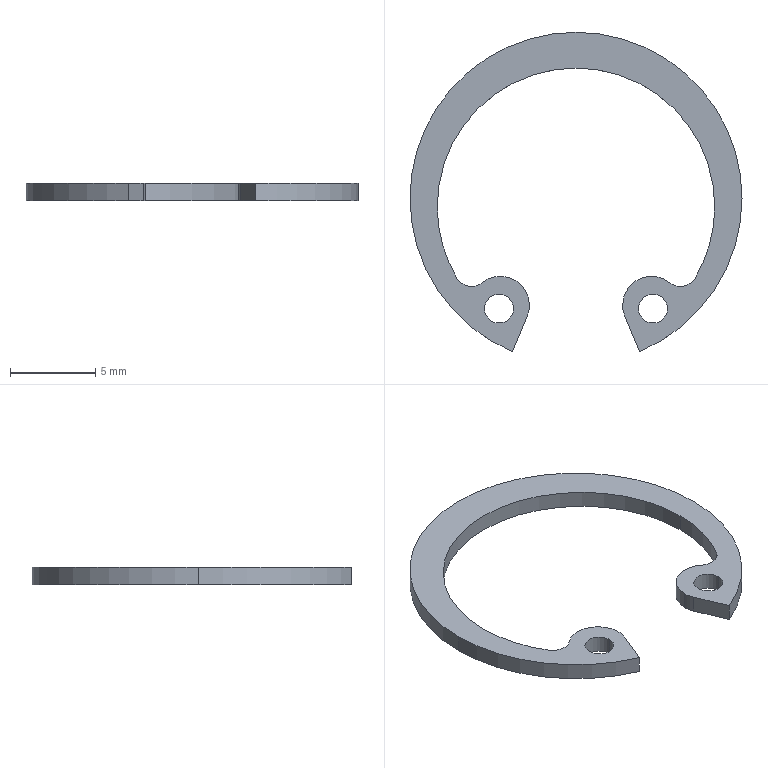Part | SolidWorks | features Extrusion 1 | 1 solid | 19 faces | box 19.5 x 18.758 x 1 mm | volume 92.859 mm3 | cylinder 15 | plane 4 | commonest cylinder face diameters 1.7 x4 3.4 x3 16.3 x3 19.5 x3 2 x2
STEP:
#1=CARTESIAN_POINT('',(3.673,-6.477,1.));
#2=VERTEX_POINT('',#1);
#3=CARTESIAN_POINT('',(5.373,-6.477,1.));
#4=VERTEX_POINT('',#3);
#5=CARTESIAN_POINT('',(4.523,-6.477,1.));
#6=DIRECTION('',(0.,0.,1.));
#7=DIRECTION('',(-1.,0.,0.));
#8=AXIS2_PLACEMENT_3D('',#5,#6,#7);
#9=CIRCLE('',#8,0.85);
#10=EDGE_CURVE('',#2,#4,#9,.T.);
#11=ORIENTED_EDGE('',*,*,#10,.T.);
#12=CARTESIAN_POINT('',(5.373,-6.477,0.));
#13=VERTEX_POINT('',#12);
#14=CARTESIAN_POINT('',(5.373,-6.477,1.));
#15=DIRECTION('',(0.,0.,-1.));
#16=VECTOR('',#15,1000.);
#17=LINE('',#14,#16);
#18=EDGE_CURVE('',#4,#13,#17,.T.);
#19=ORIENTED_EDGE('',*,*,#18,.T.);
#20=CARTESIAN_POINT('',(3.673,-6.477,0.));
#21=VERTEX_POINT('',#20);
#22=CARTESIAN_POINT('',(4.523,-6.477,0.));
#23=DIRECTION('',(0.,0.,1.));
#24=DIRECTION('',(-1.,0.,0.));
#25=AXIS2_PLACEMENT_3D('',#22,#23,#24);
#26=CIRCLE('',#25,0.85);
#27=EDGE_CURVE('',#21,#13,#26,.T.);
#28=ORIENTED_EDGE('',*,*,#27,.F.);
#29=CARTESIAN_POINT('',(3.673,-6.477,1.));
#30=DIRECTION('',(0.,0.,-1.));
#31=VECTOR('',#30,1000.);
#32=LINE('',#29,#31);
#33=EDGE_CURVE('',#2,#21,#32,.T.);
#34=ORIENTED_EDGE('',*,*,#33,.F.);
#35=EDGE_LOOP('',(#11,#19,#28,#34));
#36=FACE_OUTER_BOUND('',#35,.T.);
#37=CARTESIAN_POINT('',(4.523,-6.477,1.));
#38=DIRECTION('',(0.,0.,-1.));
#39=DIRECTION('',(-1.,0.,0.));
#40=AXIS2_PLACEMENT_3D('',#37,#38,#39);
#41=CYLINDRICAL_SURFACE('',#40,0.85);
#42=ADVANCED_FACE('',(#36),#41,.F.);
#43=CARTESIAN_POINT('',(-5.373,-6.477,1.));
#44=VERTEX_POINT('',#43);
#45=CARTESIAN_POINT('',(-3.673,-6.477,1.));
#46=VERTEX_POINT('',#45);
#47=CARTESIAN_POINT('',(-4.523,-6.477,1.));
#48=DIRECTION('',(0.,0.,1.));
#49=DIRECTION('',(1.,0.,0.));
#50=AXIS2_PLACEMENT_3D('',#47,#48,#49);
#51=CIRCLE('',#50,0.85);
#52=EDGE_CURVE('',#44,#46,#51,.T.);
#53=ORIENTED_EDGE('',*,*,#52,.T.);
#54=CARTESIAN_POINT('',(-3.673,-6.477,0.));
#55=VERTEX_POINT('',#54);
#56=CARTESIAN_POINT('',(-3.673,-6.477,1.));
#57=DIRECTION('',(0.,0.,-1.));
#58=VECTOR('',#57,1000.);
#59=LINE('',#56,#58);
#60=EDGE_CURVE('',#46,#55,#59,.T.);
#61=ORIENTED_EDGE('',*,*,#60,.T.);
#62=CARTESIAN_POINT('',(-5.373,-6.477,0.));
#63=VERTEX_POINT('',#62);
#64=CARTESIAN_POINT('',(-4.523,-6.477,0.));
#65=DIRECTION('',(0.,0.,1.));
#66=DIRECTION('',(1.,0.,0.));
#67=AXIS2_PLACEMENT_3D('',#64,#65,#66);
#68=CIRCLE('',#67,0.85);
#69=EDGE_CURVE('',#63,#55,#68,.T.);
#70=ORIENTED_EDGE('',*,*,#69,.F.);
#71=CARTESIAN_POINT('',(-5.373,-6.477,1.));
#72=DIRECTION('',(0.,0.,-1.));
#73=VECTOR('',#72,1000.);
#74=LINE('',#71,#73);
#75=EDGE_CURVE('',#44,#63,#74,.T.);
#76=ORIENTED_EDGE('',*,*,#75,.F.);
#77=EDGE_LOOP('',(#53,#61,#70,#76));
#78=FACE_OUTER_BOUND('',#77,.T.);
#79=CARTESIAN_POINT('',(-4.523,-6.477,1.));
#80=DIRECTION('',(0.,0.,-1.));
#81=DIRECTION('',(-1.,0.,0.));
#82=AXIS2_PLACEMENT_3D('',#79,#80,#81);
#83=CYLINDRICAL_SURFACE('',#82,0.85);
#84=ADVANCED_FACE('',(#78),#83,.F.);
#85=CARTESIAN_POINT('',(9.75,0.,1.));
#86=VERTEX_POINT('',#85);
#87=CARTESIAN_POINT('',(-9.75,0.,1.));
#88=VERTEX_POINT('',#87);
#89=CARTESIAN_POINT('',(0.,0.,1.));
#90=DIRECTION('',(0.,0.,1.));
#91=DIRECTION('',(1.,0.,0.));
#92=AXIS2_PLACEMENT_3D('',#89,#90,#91);
#93=CIRCLE('',#92,9.75);
#94=EDGE_CURVE('',#86,#88,#93,.T.);
#95=ORIENTED_EDGE('',*,*,#94,.F.);
#96=CARTESIAN_POINT('',(9.75,0.,0.));
#97=VERTEX_POINT('',#96);
#98=CARTESIAN_POINT('',(9.75,0.,1.));
#99=DIRECTION('',(0.,0.,-1.));
#100=VECTOR('',#99,1000.);
#101=LINE('',#98,#100);
#102=EDGE_CURVE('',#86,#97,#101,.T.);
#103=ORIENTED_EDGE('',*,*,#102,.T.);
#104=CARTESIAN_POINT('',(-9.75,0.,0.));
#105=VERTEX_POINT('',#104);
#106=CARTESIAN_POINT('',(0.,0.,0.));
#107=DIRECTION('',(0.,0.,1.));
#108=DIRECTION('',(1.,0.,0.));
#109=AXIS2_PLACEMENT_3D('',#106,#107,#108);
#110=CIRCLE('',#109,9.75);
#111=EDGE_CURVE('',#97,#105,#110,.T.);
#112=ORIENTED_EDGE('',*,*,#111,.T.);
#113=CARTESIAN_POINT('',(-9.75,0.,1.));
#114=DIRECTION('',(0.,0.,-1.));
#115=VECTOR('',#114,1000.);
#116=LINE('',#113,#115);
#117=EDGE_CURVE('',#88,#105,#116,.T.);
#118=ORIENTED_EDGE('',*,*,#117,.F.);
#119=EDGE_LOOP('',(#95,#103,#112,#118));
#120=FACE_OUTER_BOUND('',#119,.T.);
#121=CARTESIAN_POINT('',(0.,0.,1.));
#122=DIRECTION('',(0.,0.,-1.));
#123=DIRECTION('',(-1.,0.,0.));
#124=AXIS2_PLACEMENT_3D('',#121,#122,#123);
#125=CYLINDRICAL_SURFACE('',#124,9.75);
#126=ADVANCED_FACE('',(#120),#125,.T.);
#127=CARTESIAN_POINT('',(-3.731,-9.008,1.));
#128=VERTEX_POINT('',#127);
#129=CARTESIAN_POINT('',(0.,0.,1.));
#130=DIRECTION('',(0.,0.,1.));
#131=DIRECTION('',(1.,0.,0.));
#132=AXIS2_PLACEMENT_3D('',#129,#130,#131);
#133=CIRCLE('',#132,9.75);
#134=EDGE_CURVE('',#88,#128,#133,.T.);
#135=ORIENTED_EDGE('',*,*,#134,.F.);
#136=ORIENTED_EDGE('',*,*,#117,.T.);
#137=CARTESIAN_POINT('',(-3.731,-9.008,0.));
#138=VERTEX_POINT('',#137);
#139=CARTESIAN_POINT('',(0.,0.,0.));
#140=DIRECTION('',(0.,0.,1.));
#141=DIRECTION('',(1.,0.,0.));
#142=AXIS2_PLACEMENT_3D('',#139,#140,#141);
#143=CIRCLE('',#142,9.75);
#144=EDGE_CURVE('',#105,#138,#143,.T.);
#145=ORIENTED_EDGE('',*,*,#144,.T.);
#146=CARTESIAN_POINT('',(-3.731,-9.008,1.));
#147=DIRECTION('',(0.,0.,-1.));
#148=VECTOR('',#147,1000.);
#149=LINE('',#146,#148);
#150=EDGE_CURVE('',#128,#138,#149,.T.);
#151=ORIENTED_EDGE('',*,*,#150,.F.);
#152=EDGE_LOOP('',(#135,#136,#145,#151));
#153=FACE_OUTER_BOUND('',#152,.T.);
#154=CARTESIAN_POINT('',(0.,0.,1.));
#155=DIRECTION('',(0.,0.,-1.));
#156=DIRECTION('',(-1.,0.,0.));
#157=AXIS2_PLACEMENT_3D('',#154,#155,#156);
#158=CYLINDRICAL_SURFACE('',#157,9.75);
#159=ADVANCED_FACE('',(#153),#158,.T.);
#160=CARTESIAN_POINT('',(2.741,-6.278,1.));
#161=VERTEX_POINT('',#160);
#162=CARTESIAN_POINT('',(2.87,-6.929,1.));
#163=VERTEX_POINT('',#162);
#164=CARTESIAN_POINT('',(4.441,-6.278,1.));
#165=DIRECTION('',(0.,0.,1.));
#166=DIRECTION('',(-1.,0.,0.));
#167=AXIS2_PLACEMENT_3D('',#164,#165,#166);
#168=CIRCLE('',#167,1.7);
#169=EDGE_CURVE('',#161,#163,#168,.T.);
#170=ORIENTED_EDGE('',*,*,#169,.F.);
#171=CARTESIAN_POINT('',(2.741,-6.278,0.));
#172=VERTEX_POINT('',#171);
#173=CARTESIAN_POINT('',(2.741,-6.278,1.));
#174=DIRECTION('',(0.,0.,-1.));
#175=VECTOR('',#174,1000.);
#176=LINE('',#173,#175);
#177=EDGE_CURVE('',#161,#172,#176,.T.);
#178=ORIENTED_EDGE('',*,*,#177,.T.);
#179=CARTESIAN_POINT('',(2.87,-6.929,0.));
#180=VERTEX_POINT('',#179);
#181=CARTESIAN_POINT('',(4.441,-6.278,0.));
#182=DIRECTION('',(0.,0.,1.));
#183=DIRECTION('',(-1.,0.,0.));
#184=AXIS2_PLACEMENT_3D('',#181,#182,#183);
#185=CIRCLE('',#184,1.7);
#186=EDGE_CURVE('',#172,#180,#185,.T.);
#187=ORIENTED_EDGE('',*,*,#186,.T.);
#188=CARTESIAN_POINT('',(2.87,-6.929,1.));
#189=DIRECTION('',(0.,0.,-1.));
#190=VECTOR('',#189,1000.);
#191=LINE('',#188,#190);
#192=EDGE_CURVE('',#163,#180,#191,.T.);
#193=ORIENTED_EDGE('',*,*,#192,.F.);
#194=EDGE_LOOP('',(#170,#178,#187,#193));
#195=FACE_OUTER_BOUND('',#194,.T.);
#196=CARTESIAN_POINT('',(4.441,-6.278,1.));
#197=DIRECTION('',(0.,0.,-1.));
#198=DIRECTION('',(-1.,0.,0.));
#199=AXIS2_PLACEMENT_3D('',#196,#197,#198);
#200=CYLINDRICAL_SURFACE('',#199,1.7);
#201=ADVANCED_FACE('',(#195),#200,.T.);
#202=CARTESIAN_POINT('',(8.15,-0.5,1.));
#203=VERTEX_POINT('',#202);
#204=CARTESIAN_POINT('',(6.991,-4.689,1.));
#205=VERTEX_POINT('',#204);
#206=CARTESIAN_POINT('',(0.,-0.5,1.));
#207=DIRECTION('',(0.,0.,-1.));
#208=DIRECTION('',(1.,0.,0.));
#209=AXIS2_PLACEMENT_3D('',#206,#207,#208);
#210=CIRCLE('',#209,8.15);
#211=EDGE_CURVE('',#203,#205,#210,.T.);
#212=ORIENTED_EDGE('',*,*,#211,.F.);
#213=CARTESIAN_POINT('',(8.15,-0.5,0.));
#214=VERTEX_POINT('',#213);
#215=CARTESIAN_POINT('',(8.15,-0.5,1.));
#216=DIRECTION('',(0.,0.,-1.));
#217=VECTOR('',#216,1000.);
#218=LINE('',#215,#217);
#219=EDGE_CURVE('',#203,#214,#218,.T.);
#220=ORIENTED_EDGE('',*,*,#219,.T.);
#221=CARTESIAN_POINT('',(6.991,-4.689,0.));
#222=VERTEX_POINT('',#221);
#223=CARTESIAN_POINT('',(0.,-0.5,0.));
#224=DIRECTION('',(0.,0.,-1.));
#225=DIRECTION('',(1.,0.,0.));
#226=AXIS2_PLACEMENT_3D('',#223,#224,#225);
#227=CIRCLE('',#226,8.15);
#228=EDGE_CURVE('',#214,#222,#227,.T.);
#229=ORIENTED_EDGE('',*,*,#228,.T.);
#230=CARTESIAN_POINT('',(6.991,-4.689,1.));
#231=DIRECTION('',(0.,0.,-1.));
#232=VECTOR('',#231,1000.);
#233=LINE('',#230,#232);
#234=EDGE_CURVE('',#205,#222,#233,.T.);
#235=ORIENTED_EDGE('',*,*,#234,.F.);
#236=EDGE_LOOP('',(#212,#220,#229,#235));
#237=FACE_OUTER_BOUND('',#236,.T.);
#238=CARTESIAN_POINT('',(0.,-0.5,1.));
#239=DIRECTION('',(0.,0.,-1.));
#240=DIRECTION('',(-1.,0.,0.));
#241=AXIS2_PLACEMENT_3D('',#238,#239,#240);
#242=CYLINDRICAL_SURFACE('',#241,8.15);
#243=ADVANCED_FACE('',(#237),#242,.F.);
#244=ORIENTED_EDGE('',*,*,#219,.F.);
#245=CARTESIAN_POINT('',(-8.15,-0.5,1.));
#246=VERTEX_POINT('',#245);
#247=CARTESIAN_POINT('',(0.,-0.5,1.));
#248=DIRECTION('',(0.,0.,-1.));
#249=DIRECTION('',(1.,0.,0.));
#250=AXIS2_PLACEMENT_3D('',#247,#248,#249);
#251=CIRCLE('',#250,8.15);
#252=EDGE_CURVE('',#246,#203,#251,.T.);
#253=ORIENTED_EDGE('',*,*,#252,.F.);
#254=CARTESIAN_POINT('',(-8.15,-0.5,0.));
#255=VERTEX_POINT('',#254);
#256=CARTESIAN_POINT('',(-8.15,-0.5,1.));
#257=DIRECTION('',(0.,0.,-1.));
#258=VECTOR('',#257,1000.);
#259=LINE('',#256,#258);
#260=EDGE_CURVE('',#246,#255,#259,.T.);
#261=ORIENTED_EDGE('',*,*,#260,.T.);
#262=CARTESIAN_POINT('',(0.,-0.5,0.));
#263=DIRECTION('',(0.,0.,-1.));
#264=DIRECTION('',(1.,0.,0.));
#265=AXIS2_PLACEMENT_3D('',#262,#263,#264);
#266=CIRCLE('',#265,8.15);
#267=EDGE_CURVE('',#255,#214,#266,.T.);
#268=ORIENTED_EDGE('',*,*,#267,.T.);
#269=EDGE_LOOP('',(#244,#253,#261,#268));
#270=FACE_OUTER_BOUND('',#269,.T.);
#271=CARTESIAN_POINT('',(0.,-0.5,1.));
#272=DIRECTION('',(0.,0.,-1.));
#273=DIRECTION('',(-1.,0.,0.));
#274=AXIS2_PLACEMENT_3D('',#271,#272,#273);
#275=CYLINDRICAL_SURFACE('',#274,8.15);
#276=ADVANCED_FACE('',(#270),#275,.F.);
#277=ORIENTED_EDGE('',*,*,#52,.F.);
#278=CARTESIAN_POINT('',(-4.523,-6.477,1.));
#279=DIRECTION('',(0.,0.,1.));
#280=DIRECTION('',(1.,0.,0.));
#281=AXIS2_PLACEMENT_3D('',#278,#279,#280);
#282=CIRCLE('',#281,0.85);
#283=EDGE_CURVE('',#46,#44,#282,.T.);
#284=ORIENTED_EDGE('',*,*,#283,.F.);
#285=EDGE_LOOP('',(#277,#284));
#286=FACE_BOUND('',#285,.T.);
#287=CARTESIAN_POINT('',(-2.87,-6.929,1.));
#288=VERTEX_POINT('',#287);
#289=CARTESIAN_POINT('',(-5.506,-4.954,1.));
#290=VERTEX_POINT('',#289);
#291=CARTESIAN_POINT('',(-4.441,-6.278,1.));
#292=DIRECTION('',(0.,0.,1.));
#293=DIRECTION('',(1.,0.,0.));
#294=AXIS2_PLACEMENT_3D('',#291,#292,#293);
#295=CIRCLE('',#294,1.7);
#296=EDGE_CURVE('',#288,#290,#295,.T.);
#297=ORIENTED_EDGE('',*,*,#296,.T.);
#298=CARTESIAN_POINT('',(-6.991,-4.689,1.));
#299=VERTEX_POINT('',#298);
#300=CARTESIAN_POINT('',(-6.133,-4.175,1.));
#301=DIRECTION('',(0.,0.,-1.));
#302=DIRECTION('',(-1.,0.,0.));
#303=AXIS2_PLACEMENT_3D('',#300,#301,#302);
#304=CIRCLE('',#303,1.);
#305=EDGE_CURVE('',#290,#299,#304,.T.);
#306=ORIENTED_EDGE('',*,*,#305,.T.);
#307=CARTESIAN_POINT('',(0.,-0.5,1.));
#308=DIRECTION('',(0.,0.,-1.));
#309=DIRECTION('',(1.,0.,0.));
#310=AXIS2_PLACEMENT_3D('',#307,#308,#309);
#311=CIRCLE('',#310,8.15);
#312=EDGE_CURVE('',#299,#246,#311,.T.);
#313=ORIENTED_EDGE('',*,*,#312,.T.);
#314=ORIENTED_EDGE('',*,*,#252,.T.);
#315=ORIENTED_EDGE('',*,*,#211,.T.);
#316=CARTESIAN_POINT('',(5.506,-4.954,1.));
#317=VERTEX_POINT('',#316);
#318=CARTESIAN_POINT('',(6.133,-4.175,1.));
#319=DIRECTION('',(0.,0.,-1.));
#320=DIRECTION('',(1.,0.,0.));
#321=AXIS2_PLACEMENT_3D('',#318,#319,#320);
#322=CIRCLE('',#321,1.);
#323=EDGE_CURVE('',#205,#317,#322,.T.);
#324=ORIENTED_EDGE('',*,*,#323,.T.);
#325=CARTESIAN_POINT('',(4.441,-6.278,1.));
#326=DIRECTION('',(0.,0.,1.));
#327=DIRECTION('',(-1.,0.,0.));
#328=AXIS2_PLACEMENT_3D('',#325,#326,#327);
#329=CIRCLE('',#328,1.7);
#330=EDGE_CURVE('',#317,#161,#329,.T.);
#331=ORIENTED_EDGE('',*,*,#330,.T.);
#332=ORIENTED_EDGE('',*,*,#169,.T.);
#333=CARTESIAN_POINT('',(3.731,-9.008,1.));
#334=VERTEX_POINT('',#333);
#335=CARTESIAN_POINT('',(2.87,-6.929,1.));
#336=DIRECTION('',(0.3827,-0.9239,0.));
#337=VECTOR('',#336,1000.);
#338=LINE('',#335,#337);
#339=EDGE_CURVE('',#163,#334,#338,.T.);
#340=ORIENTED_EDGE('',*,*,#339,.T.);
#341=CARTESIAN_POINT('',(0.,0.,1.));
#342=DIRECTION('',(0.,0.,1.));
#343=DIRECTION('',(1.,0.,0.));
#344=AXIS2_PLACEMENT_3D('',#341,#342,#343);
#345=CIRCLE('',#344,9.75);
#346=EDGE_CURVE('',#334,#86,#345,.T.);
#347=ORIENTED_EDGE('',*,*,#346,.T.);
#348=ORIENTED_EDGE('',*,*,#94,.T.);
#349=ORIENTED_EDGE('',*,*,#134,.T.);
#350=CARTESIAN_POINT('',(-2.87,-6.929,1.));
#351=DIRECTION('',(0.3827,0.9239,0.));
#352=VECTOR('',#351,1000.);
#353=LINE('',#350,#352);
#354=EDGE_CURVE('',#128,#288,#353,.T.);
#355=ORIENTED_EDGE('',*,*,#354,.T.);
#356=EDGE_LOOP('',(#297,#306,#313,#314,#315,#324,#331,#332,#340,#347,#348,#349,#355));
#357=FACE_OUTER_BOUND('',#356,.T.);
#358=ORIENTED_EDGE('',*,*,#10,.F.);
#359=CARTESIAN_POINT('',(4.523,-6.477,1.));
#360=DIRECTION('',(0.,0.,1.));
#361=DIRECTION('',(-1.,0.,0.));
#362=AXIS2_PLACEMENT_3D('',#359,#360,#361);
#363=CIRCLE('',#362,0.85);
#364=EDGE_CURVE('',#4,#2,#363,.T.);
#365=ORIENTED_EDGE('',*,*,#364,.F.);
#366=EDGE_LOOP('',(#358,#365));
#367=FACE_BOUND('',#366,.T.);
#368=CARTESIAN_POINT('',(-4.441,-6.278,1.));
#369=DIRECTION('',(0.,0.,1.));
#370=DIRECTION('',(1.,0.,0.));
#371=AXIS2_PLACEMENT_3D('',#368,#369,#370);
#372=PLANE('',#371);
#373=ADVANCED_FACE('',(#286,#357,#367),#372,.T.);
#374=CARTESIAN_POINT('',(-2.87,-6.929,0.));
#375=VERTEX_POINT('',#374);
#376=CARTESIAN_POINT('',(-5.506,-4.954,0.));
#377=VERTEX_POINT('',#376);
#378=CARTESIAN_POINT('',(-4.441,-6.278,0.));
#379=DIRECTION('',(0.,0.,1.));
#380=DIRECTION('',(1.,0.,0.));
#381=AXIS2_PLACEMENT_3D('',#378,#379,#380);
#382=CIRCLE('',#381,1.7);
#383=EDGE_CURVE('',#375,#377,#382,.T.);
#384=ORIENTED_EDGE('',*,*,#383,.F.);
#385=CARTESIAN_POINT('',(-2.87,-6.929,0.));
#386=DIRECTION('',(0.3827,0.9239,0.));
#387=VECTOR('',#386,1000.);
#388=LINE('',#385,#387);
#389=EDGE_CURVE('',#138,#375,#388,.T.);
#390=ORIENTED_EDGE('',*,*,#389,.F.);
#391=ORIENTED_EDGE('',*,*,#144,.F.);
#392=ORIENTED_EDGE('',*,*,#111,.F.);
#393=CARTESIAN_POINT('',(3.731,-9.008,0.));
#394=VERTEX_POINT('',#393);
#395=CARTESIAN_POINT('',(0.,0.,0.));
#396=DIRECTION('',(0.,0.,1.));
#397=DIRECTION('',(1.,0.,0.));
#398=AXIS2_PLACEMENT_3D('',#395,#396,#397);
#399=CIRCLE('',#398,9.75);
#400=EDGE_CURVE('',#394,#97,#399,.T.);
#401=ORIENTED_EDGE('',*,*,#400,.F.);
#402=CARTESIAN_POINT('',(2.87,-6.929,0.));
#403=DIRECTION('',(0.3827,-0.9239,0.));
#404=VECTOR('',#403,1000.);
#405=LINE('',#402,#404);
#406=EDGE_CURVE('',#180,#394,#405,.T.);
#407=ORIENTED_EDGE('',*,*,#406,.F.);
#408=ORIENTED_EDGE('',*,*,#186,.F.);
#409=CARTESIAN_POINT('',(5.506,-4.954,0.));
#410=VERTEX_POINT('',#409);
#411=CARTESIAN_POINT('',(4.441,-6.278,0.));
#412=DIRECTION('',(0.,0.,1.));
#413=DIRECTION('',(-1.,0.,0.));
#414=AXIS2_PLACEMENT_3D('',#411,#412,#413);
#415=CIRCLE('',#414,1.7);
#416=EDGE_CURVE('',#410,#172,#415,.T.);
#417=ORIENTED_EDGE('',*,*,#416,.F.);
#418=CARTESIAN_POINT('',(6.133,-4.175,0.));
#419=DIRECTION('',(0.,0.,-1.));
#420=DIRECTION('',(1.,0.,0.));
#421=AXIS2_PLACEMENT_3D('',#418,#419,#420);
#422=CIRCLE('',#421,1.);
#423=EDGE_CURVE('',#222,#410,#422,.T.);
#424=ORIENTED_EDGE('',*,*,#423,.F.);
#425=ORIENTED_EDGE('',*,*,#228,.F.);
#426=ORIENTED_EDGE('',*,*,#267,.F.);
#427=CARTESIAN_POINT('',(-6.991,-4.689,0.));
#428=VERTEX_POINT('',#427);
#429=CARTESIAN_POINT('',(0.,-0.5,0.));
#430=DIRECTION('',(0.,0.,-1.));
#431=DIRECTION('',(1.,0.,0.));
#432=AXIS2_PLACEMENT_3D('',#429,#430,#431);
#433=CIRCLE('',#432,8.15);
#434=EDGE_CURVE('',#428,#255,#433,.T.);
#435=ORIENTED_EDGE('',*,*,#434,.F.);
#436=CARTESIAN_POINT('',(-6.133,-4.175,0.));
#437=DIRECTION('',(0.,0.,-1.));
#438=DIRECTION('',(-1.,0.,0.));
#439=AXIS2_PLACEMENT_3D('',#436,#437,#438);
#440=CIRCLE('',#439,1.);
#441=EDGE_CURVE('',#377,#428,#440,.T.);
#442=ORIENTED_EDGE('',*,*,#441,.F.);
#443=EDGE_LOOP('',(#384,#390,#391,#392,#401,#407,#408,#417,#424,#425,#426,#435,#442));
#444=FACE_OUTER_BOUND('',#443,.T.);
#445=ORIENTED_EDGE('',*,*,#69,.T.);
#446=CARTESIAN_POINT('',(-4.523,-6.477,0.));
#447=DIRECTION('',(0.,0.,1.));
#448=DIRECTION('',(1.,0.,0.));
#449=AXIS2_PLACEMENT_3D('',#446,#447,#448);
#450=CIRCLE('',#449,0.85);
#451=EDGE_CURVE('',#55,#63,#450,.T.);
#452=ORIENTED_EDGE('',*,*,#451,.T.);
#453=EDGE_LOOP('',(#445,#452));
#454=FACE_BOUND('',#453,.T.);
#455=ORIENTED_EDGE('',*,*,#27,.T.);
#456=CARTESIAN_POINT('',(4.523,-6.477,0.));
#457=DIRECTION('',(0.,0.,1.));
#458=DIRECTION('',(-1.,0.,0.));
#459=AXIS2_PLACEMENT_3D('',#456,#457,#458);
#460=CIRCLE('',#459,0.85);
#461=EDGE_CURVE('',#13,#21,#460,.T.);
#462=ORIENTED_EDGE('',*,*,#461,.T.);
#463=EDGE_LOOP('',(#455,#462));
#464=FACE_BOUND('',#463,.T.);
#465=CARTESIAN_POINT('',(-4.441,-6.278,0.));
#466=DIRECTION('',(0.,0.,1.));
#467=DIRECTION('',(1.,0.,0.));
#468=AXIS2_PLACEMENT_3D('',#465,#466,#467);
#469=PLANE('',#468);
#470=ADVANCED_FACE('',(#444,#454,#464),#469,.F.);
#471=ORIENTED_EDGE('',*,*,#383,.T.);
#472=CARTESIAN_POINT('',(-5.506,-4.954,1.));
#473=DIRECTION('',(0.,0.,-1.));
#474=VECTOR('',#473,1000.);
#475=LINE('',#472,#474);
#476=EDGE_CURVE('',#290,#377,#475,.T.);
#477=ORIENTED_EDGE('',*,*,#476,.F.);
#478=ORIENTED_EDGE('',*,*,#296,.F.);
#479=CARTESIAN_POINT('',(-2.87,-6.929,1.));
#480=DIRECTION('',(0.,0.,-1.));
#481=VECTOR('',#480,1000.);
#482=LINE('',#479,#481);
#483=EDGE_CURVE('',#288,#375,#482,.T.);
#484=ORIENTED_EDGE('',*,*,#483,.T.);
#485=EDGE_LOOP('',(#471,#477,#478,#484));
#486=FACE_OUTER_BOUND('',#485,.T.);
#487=CARTESIAN_POINT('',(-4.441,-6.278,1.));
#488=DIRECTION('',(0.,0.,-1.));
#489=DIRECTION('',(-1.,0.,0.));
#490=AXIS2_PLACEMENT_3D('',#487,#488,#489);
#491=CYLINDRICAL_SURFACE('',#490,1.7);
#492=ADVANCED_FACE('',(#486),#491,.T.);
#493=ORIENTED_EDGE('',*,*,#441,.T.);
#494=CARTESIAN_POINT('',(-6.991,-4.689,1.));
#495=DIRECTION('',(0.,0.,-1.));
#496=VECTOR('',#495,1000.);
#497=LINE('',#494,#496);
#498=EDGE_CURVE('',#299,#428,#497,.T.);
#499=ORIENTED_EDGE('',*,*,#498,.F.);
#500=ORIENTED_EDGE('',*,*,#305,.F.);
#501=ORIENTED_EDGE('',*,*,#476,.T.);
#502=EDGE_LOOP('',(#493,#499,#500,#501));
#503=FACE_OUTER_BOUND('',#502,.T.);
#504=CARTESIAN_POINT('',(-6.133,-4.175,1.));
#505=DIRECTION('',(0.,0.,-1.));
#506=DIRECTION('',(-1.,0.,0.));
#507=AXIS2_PLACEMENT_3D('',#504,#505,#506);
#508=CYLINDRICAL_SURFACE('',#507,1.);
#509=ADVANCED_FACE('',(#503),#508,.F.);
#510=ORIENTED_EDGE('',*,*,#260,.F.);
#511=ORIENTED_EDGE('',*,*,#312,.F.);
#512=ORIENTED_EDGE('',*,*,#498,.T.);
#513=ORIENTED_EDGE('',*,*,#434,.T.);
#514=EDGE_LOOP('',(#510,#511,#512,#513));
#515=FACE_OUTER_BOUND('',#514,.T.);
#516=CARTESIAN_POINT('',(0.,-0.5,1.));
#517=DIRECTION('',(0.,0.,-1.));
#518=DIRECTION('',(-1.,0.,0.));
#519=AXIS2_PLACEMENT_3D('',#516,#517,#518);
#520=CYLINDRICAL_SURFACE('',#519,8.15);
#521=ADVANCED_FACE('',(#515),#520,.F.);
#522=ORIENTED_EDGE('',*,*,#423,.T.);
#523=CARTESIAN_POINT('',(5.506,-4.954,1.));
#524=DIRECTION('',(0.,0.,-1.));
#525=VECTOR('',#524,1000.);
#526=LINE('',#523,#525);
#527=EDGE_CURVE('',#317,#410,#526,.T.);
#528=ORIENTED_EDGE('',*,*,#527,.F.);
#529=ORIENTED_EDGE('',*,*,#323,.F.);
#530=ORIENTED_EDGE('',*,*,#234,.T.);
#531=EDGE_LOOP('',(#522,#528,#529,#530));
#532=FACE_OUTER_BOUND('',#531,.T.);
#533=CARTESIAN_POINT('',(6.133,-4.175,1.));
#534=DIRECTION('',(0.,0.,-1.));
#535=DIRECTION('',(-1.,0.,0.));
#536=AXIS2_PLACEMENT_3D('',#533,#534,#535);
#537=CYLINDRICAL_SURFACE('',#536,1.);
#538=ADVANCED_FACE('',(#532),#537,.F.);
#539=ORIENTED_EDGE('',*,*,#177,.F.);
#540=ORIENTED_EDGE('',*,*,#330,.F.);
#541=ORIENTED_EDGE('',*,*,#527,.T.);
#542=ORIENTED_EDGE('',*,*,#416,.T.);
#543=EDGE_LOOP('',(#539,#540,#541,#542));
#544=FACE_OUTER_BOUND('',#543,.T.);
#545=CARTESIAN_POINT('',(4.441,-6.278,1.));
#546=DIRECTION('',(0.,0.,-1.));
#547=DIRECTION('',(-1.,0.,0.));
#548=AXIS2_PLACEMENT_3D('',#545,#546,#547);
#549=CYLINDRICAL_SURFACE('',#548,1.7);
#550=ADVANCED_FACE('',(#544),#549,.T.);
#551=ORIENTED_EDGE('',*,*,#406,.T.);
#552=CARTESIAN_POINT('',(3.731,-9.008,1.));
#553=DIRECTION('',(0.,0.,-1.));
#554=VECTOR('',#553,1000.);
#555=LINE('',#552,#554);
#556=EDGE_CURVE('',#334,#394,#555,.T.);
#557=ORIENTED_EDGE('',*,*,#556,.F.);
#558=ORIENTED_EDGE('',*,*,#339,.F.);
#559=ORIENTED_EDGE('',*,*,#192,.T.);
#560=EDGE_LOOP('',(#551,#557,#558,#559));
#561=FACE_OUTER_BOUND('',#560,.T.);
#562=CARTESIAN_POINT('',(2.87,-6.929,1.));
#563=DIRECTION('',(0.9239,0.3827,0.));
#564=DIRECTION('',(-0.3827,0.9239,0.));
#565=AXIS2_PLACEMENT_3D('',#562,#563,#564);
#566=PLANE('',#565);
#567=ADVANCED_FACE('',(#561),#566,.F.);
#568=ORIENTED_EDGE('',*,*,#102,.F.);
#569=ORIENTED_EDGE('',*,*,#346,.F.);
#570=ORIENTED_EDGE('',*,*,#556,.T.);
#571=ORIENTED_EDGE('',*,*,#400,.T.);
#572=EDGE_LOOP('',(#568,#569,#570,#571));
#573=FACE_OUTER_BOUND('',#572,.T.);
#574=CARTESIAN_POINT('',(0.,0.,1.));
#575=DIRECTION('',(0.,0.,-1.));
#576=DIRECTION('',(-1.,0.,0.));
#577=AXIS2_PLACEMENT_3D('',#574,#575,#576);
#578=CYLINDRICAL_SURFACE('',#577,9.75);
#579=ADVANCED_FACE('',(#573),#578,.T.);
#580=ORIENTED_EDGE('',*,*,#389,.T.);
#581=ORIENTED_EDGE('',*,*,#483,.F.);
#582=ORIENTED_EDGE('',*,*,#354,.F.);
#583=ORIENTED_EDGE('',*,*,#150,.T.);
#584=EDGE_LOOP('',(#580,#581,#582,#583));
#585=FACE_OUTER_BOUND('',#584,.T.);
#586=CARTESIAN_POINT('',(-2.87,-6.929,1.));
#587=DIRECTION('',(-0.9239,0.3827,0.));
#588=DIRECTION('',(-0.3827,-0.9239,0.));
#589=AXIS2_PLACEMENT_3D('',#586,#587,#588);
#590=PLANE('',#589);
#591=ADVANCED_FACE('',(#585),#590,.F.);
#592=ORIENTED_EDGE('',*,*,#60,.F.);
#593=ORIENTED_EDGE('',*,*,#283,.T.);
#594=ORIENTED_EDGE('',*,*,#75,.T.);
#595=ORIENTED_EDGE('',*,*,#451,.F.);
#596=EDGE_LOOP('',(#592,#593,#594,#595));
#597=FACE_OUTER_BOUND('',#596,.T.);
#598=CARTESIAN_POINT('',(-4.523,-6.477,1.));
#599=DIRECTION('',(0.,0.,-1.));
#600=DIRECTION('',(-1.,0.,0.));
#601=AXIS2_PLACEMENT_3D('',#598,#599,#600);
#602=CYLINDRICAL_SURFACE('',#601,0.85);
#603=ADVANCED_FACE('',(#597),#602,.F.);
#604=ORIENTED_EDGE('',*,*,#18,.F.);
#605=ORIENTED_EDGE('',*,*,#364,.T.);
#606=ORIENTED_EDGE('',*,*,#33,.T.);
#607=ORIENTED_EDGE('',*,*,#461,.F.);
#608=EDGE_LOOP('',(#604,#605,#606,#607));
#609=FACE_OUTER_BOUND('',#608,.T.);
#610=CARTESIAN_POINT('',(4.523,-6.477,1.));
#611=DIRECTION('',(0.,0.,-1.));
#612=DIRECTION('',(-1.,0.,0.));
#613=AXIS2_PLACEMENT_3D('',#610,#611,#612);
#614=CYLINDRICAL_SURFACE('',#613,0.85);
#615=ADVANCED_FACE('',(#609),#614,.F.);
#616=CLOSED_SHELL('',(#42,#84,#126,#159,#201,#243,#276,#373,#470,#492,#509,#521,#538,#550,#567,#579,#591,#603,#615));
#617=MANIFOLD_SOLID_BREP('',#616);
#618=CARTESIAN_POINT('',(0.,0.,0.));
#619=DIRECTION('',(0.,0.,1.));
#620=DIRECTION('',(1.,0.,0.));
#621=AXIS2_PLACEMENT_3D('',#618,#619,#620);
#622=(LENGTH_UNIT()NAMED_UNIT(*)SI_UNIT(.MILLI.,.METRE.));
#623=UNCERTAINTY_MEASURE_WITH_UNIT(LENGTH_MEASURE(0.00001),#622,'','');
#624=(NAMED_UNIT(*)PLANE_ANGLE_UNIT()SI_UNIT($,.RADIAN.));
#625=(NAMED_UNIT(*)SI_UNIT($,.STERADIAN.)SOLID_ANGLE_UNIT());
#626=(GEOMETRIC_REPRESENTATION_CONTEXT(3)GLOBAL_UNCERTAINTY_ASSIGNED_CONTEXT((#623))GLOBAL_UNIT_ASSIGNED_CONTEXT((#622,#624,#625))REPRESENTATION_CONTEXT('',''));
#627=ADVANCED_BREP_SHAPE_REPRESENTATION('',(#617,#621),#626);